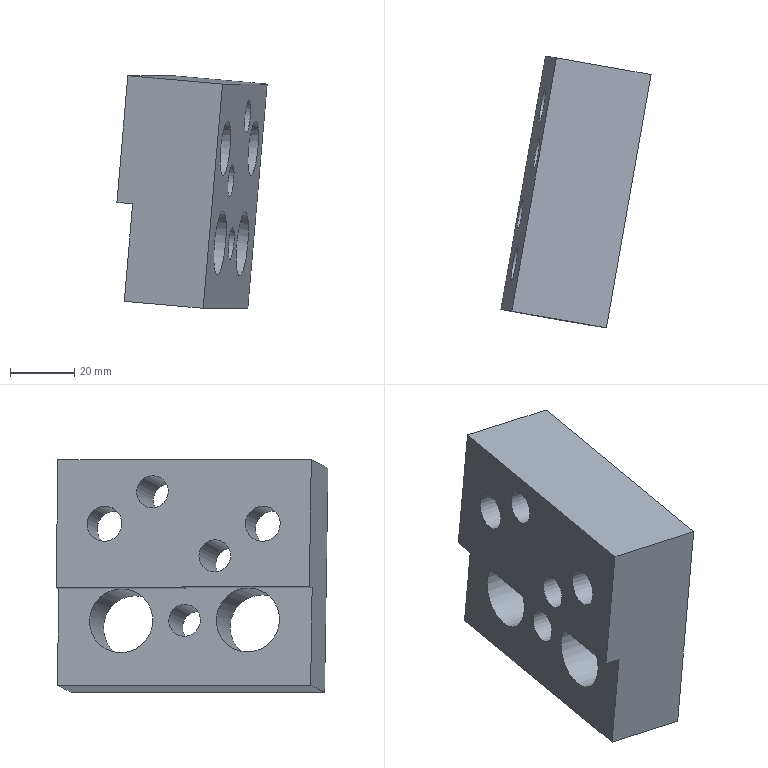Part | NX | features solid 2 | 1 solid | 21 faces | box 46.72 x 84.577 x 72.348 mm | volume 124632 mm3 | plane 11 | cylinder 10 | commonest cylinder face diameters 10 x3 11 x2 17 x2 20 x2 0.557 x1
STEP:
#1=CARTESIAN_POINT('',(413.654,2.711,48.436));
#2=VERTEX_POINT('',#1);
#3=CARTESIAN_POINT('',(412.178,-5.66,48.436));
#4=DIRECTION('',(0.9811,-0.173,-0.08716));
#5=DIRECTION('',(0.1736,0.9848,0.));
#6=AXIS2_PLACEMENT_3D('',#3,#4,#5);
#7=CIRCLE('',#6,8.5);
#8=EDGE_CURVE('',#2,#2,#7,.F.);
#9=ORIENTED_EDGE('',*,*,#8,.T.);
#10=EDGE_LOOP('',(#9));
#11=FACE_BOUND('',#10,.T.);
#12=CARTESIAN_POINT('',(422.336,51.951,48.436));
#13=VERTEX_POINT('',#12);
#14=CARTESIAN_POINT('',(420.86,43.58,48.436));
#15=DIRECTION('',(0.9811,-0.173,-0.08716));
#16=DIRECTION('',(0.1736,0.9848,0.));
#17=AXIS2_PLACEMENT_3D('',#14,#15,#16);
#18=CIRCLE('',#17,8.5);
#19=EDGE_CURVE('',#13,#13,#18,.F.);
#20=ORIENTED_EDGE('',*,*,#19,.T.);
#21=EDGE_LOOP('',(#20));
#22=FACE_BOUND('',#21,.T.);
#23=CARTESIAN_POINT('',(414.863,24.481,18.839));
#24=VERTEX_POINT('',#23);
#25=CARTESIAN_POINT('',(413.995,19.557,18.839));
#26=DIRECTION('',(0.9811,-0.173,-0.08716));
#27=DIRECTION('',(0.1736,0.9848,0.));
#28=AXIS2_PLACEMENT_3D('',#25,#26,#27);
#29=CIRCLE('',#28,5.);
#30=EDGE_CURVE('',#24,#24,#29,.T.);
#31=ORIENTED_EDGE('',*,*,#30,.F.);
#32=EDGE_LOOP('',(#31));
#33=FACE_BOUND('',#32,.T.);
#34=CARTESIAN_POINT('',(425.182,58.05,68.36));
#35=VERTEX_POINT('',#34);
#36=CARTESIAN_POINT('',(411.29,-20.735,68.36));
#37=VERTEX_POINT('',#36);
#38=CARTESIAN_POINT('',(425.182,58.05,68.36));
#39=DIRECTION('',(0.1736,0.9848,0.));
#40=VECTOR('',#39,1000.);
#41=LINE('',#38,#40);
#42=EDGE_CURVE('',#35,#37,#41,.F.);
#43=ORIENTED_EDGE('',*,*,#42,.T.);
#44=CARTESIAN_POINT('',(405.282,-19.675,-1.373));
#45=VERTEX_POINT('',#44);
#46=CARTESIAN_POINT('',(412.427,-20.935,81.56));
#47=DIRECTION('',(-0.08583,0.01513,-0.9962));
#48=VECTOR('',#47,1000.);
#49=LINE('',#46,#48);
#50=EDGE_CURVE('',#45,#37,#49,.F.);
#51=ORIENTED_EDGE('',*,*,#50,.F.);
#52=CARTESIAN_POINT('',(419.174,59.109,-1.373));
#53=VERTEX_POINT('',#52);
#54=CARTESIAN_POINT('',(419.174,59.109,-1.373));
#55=DIRECTION('',(0.1736,0.9848,0.));
#56=VECTOR('',#55,1000.);
#57=LINE('',#54,#56);
#58=EDGE_CURVE('',#45,#53,#57,.T.);
#59=ORIENTED_EDGE('',*,*,#58,.T.);
#60=CARTESIAN_POINT('',(421.813,58.644,29.261));
#61=DIRECTION('',(-0.08583,0.01513,-0.9962));
#62=VECTOR('',#61,1000.);
#63=LINE('',#60,#62);
#64=EDGE_CURVE('',#35,#53,#63,.T.);
#65=ORIENTED_EDGE('',*,*,#64,.F.);
#66=EDGE_LOOP('',(#43,#51,#59,#65));
#67=FACE_BOUND('',#66,.T.);
#68=CARTESIAN_POINT('',(419.192,49.1,18.7));
#69=VERTEX_POINT('',#68);
#70=CARTESIAN_POINT('',(417.455,39.252,18.7));
#71=DIRECTION('',(0.9811,-0.173,-0.08716));
#72=DIRECTION('',(0.1736,0.9848,0.));
#73=AXIS2_PLACEMENT_3D('',#70,#71,#72);
#74=CIRCLE('',#73,10.);
#75=EDGE_CURVE('',#69,#69,#74,.T.);
#76=ORIENTED_EDGE('',*,*,#75,.F.);
#77=EDGE_LOOP('',(#76));
#78=FACE_BOUND('',#77,.T.);
#79=CARTESIAN_POINT('',(412.271,9.711,18.977));
#80=VERTEX_POINT('',#79);
#81=CARTESIAN_POINT('',(410.535,-0.137,18.977));
#82=DIRECTION('',(0.9811,-0.173,-0.08716));
#83=DIRECTION('',(0.1736,0.9848,0.));
#84=AXIS2_PLACEMENT_3D('',#81,#82,#83);
#85=CIRCLE('',#84,10.);
#86=EDGE_CURVE('',#80,#80,#85,.T.);
#87=ORIENTED_EDGE('',*,*,#86,.F.);
#88=EDGE_LOOP('',(#87));
#89=FACE_BOUND('',#88,.T.);
#90=CARTESIAN_POINT('',(419.982,33.581,58.398));
#91=VERTEX_POINT('',#90);
#92=CARTESIAN_POINT('',(419.114,28.657,58.398));
#93=DIRECTION('',(0.9811,-0.173,-0.08716));
#94=DIRECTION('',(0.1736,0.9848,0.));
#95=AXIS2_PLACEMENT_3D('',#92,#93,#94);
#96=CIRCLE('',#95,5.);
#97=EDGE_CURVE('',#91,#91,#96,.T.);
#98=ORIENTED_EDGE('',*,*,#97,.F.);
#99=EDGE_LOOP('',(#98));
#100=FACE_BOUND('',#99,.T.);
#101=CARTESIAN_POINT('',(414.793,14.188,38.474));
#102=VERTEX_POINT('',#101);
#103=CARTESIAN_POINT('',(413.924,9.264,38.474));
#104=DIRECTION('',(0.9811,-0.173,-0.08716));
#105=DIRECTION('',(0.1736,0.9848,0.));
#106=AXIS2_PLACEMENT_3D('',#103,#104,#105);
#107=CIRCLE('',#106,5.);
#108=EDGE_CURVE('',#102,#102,#107,.T.);
#109=ORIENTED_EDGE('',*,*,#108,.F.);
#110=EDGE_LOOP('',(#109));
#111=FACE_BOUND('',#110,.T.);
#112=CARTESIAN_POINT('',(426.319,57.849,81.56));
#113=DIRECTION('',(-0.9811,0.173,0.08716));
#114=DIRECTION('',(-0.1736,-0.9848,0.));
#115=AXIS2_PLACEMENT_3D('',#112,#113,#114);
#116=PLANE('',#115);
#117=ADVANCED_FACE('',(#11,#22,#33,#67,#78,#89,#100,#111),#116,.F.);
#118=CARTESIAN_POINT('',(385.361,19.377,41.089));
#119=VERTEX_POINT('',#118);
#120=CARTESIAN_POINT('',(384.493,14.453,41.089));
#121=DIRECTION('',(0.9811,-0.173,-0.08716));
#122=DIRECTION('',(0.1736,0.9848,0.));
#123=AXIS2_PLACEMENT_3D('',#120,#121,#122);
#124=CIRCLE('',#123,5.);
#125=EDGE_CURVE('',#119,#119,#124,.F.);
#126=ORIENTED_EDGE('',*,*,#125,.T.);
#127=EDGE_LOOP('',(#126));
#128=FACE_BOUND('',#127,.T.);
#129=ORIENTED_EDGE('',*,*,#108,.T.);
#130=EDGE_LOOP('',(#129));
#131=FACE_BOUND('',#130,.T.);
#132=CARTESIAN_POINT('',(315.818,26.562,47.19));
#133=DIRECTION('',(0.9811,-0.173,-0.08716));
#134=DIRECTION('',(-0.1736,-0.9848,0.));
#135=AXIS2_PLACEMENT_3D('',#132,#133,#134);
#136=CYLINDRICAL_SURFACE('',#135,5.);
#137=ADVANCED_FACE('',(#128,#131),#136,.F.);
#138=CARTESIAN_POINT('',(390.55,38.771,61.013));
#139=VERTEX_POINT('',#138);
#140=CARTESIAN_POINT('',(389.682,33.847,61.013));
#141=DIRECTION('',(0.9811,-0.173,-0.08716));
#142=DIRECTION('',(0.1736,0.9848,0.));
#143=AXIS2_PLACEMENT_3D('',#140,#141,#142);
#144=CIRCLE('',#143,5.);
#145=EDGE_CURVE('',#139,#139,#144,.F.);
#146=ORIENTED_EDGE('',*,*,#145,.T.);
#147=EDGE_LOOP('',(#146));
#148=FACE_BOUND('',#147,.T.);
#149=ORIENTED_EDGE('',*,*,#97,.T.);
#150=EDGE_LOOP('',(#149));
#151=FACE_BOUND('',#150,.T.);
#152=CARTESIAN_POINT('',(321.008,45.956,67.114));
#153=DIRECTION('',(0.9811,-0.173,-0.08716));
#154=DIRECTION('',(-0.1736,-0.9848,0.));
#155=AXIS2_PLACEMENT_3D('',#152,#153,#154);
#156=CYLINDRICAL_SURFACE('',#155,5.);
#157=ADVANCED_FACE('',(#148,#151),#156,.F.);
#158=CARTESIAN_POINT('',(394.647,63.434,0.8055));
#159=VERTEX_POINT('',#158);
#160=CARTESIAN_POINT('',(380.755,-15.351,0.8055));
#161=VERTEX_POINT('',#160);
#162=CARTESIAN_POINT('',(394.647,63.434,0.8055));
#163=DIRECTION('',(-0.1736,-0.9848,0.));
#164=VECTOR('',#163,1000.);
#165=LINE('',#162,#164);
#166=EDGE_CURVE('',#159,#161,#165,.T.);
#167=ORIENTED_EDGE('',*,*,#166,.F.);
#168=CARTESIAN_POINT('',(419.174,59.109,-1.373));
#169=DIRECTION('',(-0.9811,0.173,0.08716));
#170=VECTOR('',#169,1000.);
#171=LINE('',#168,#170);
#172=EDGE_CURVE('',#53,#159,#171,.T.);
#173=ORIENTED_EDGE('',*,*,#172,.F.);
#174=ORIENTED_EDGE('',*,*,#58,.F.);
#175=CARTESIAN_POINT('',(405.282,-19.675,-1.373));
#176=DIRECTION('',(-0.9811,0.173,0.08716));
#177=VECTOR('',#176,1000.);
#178=LINE('',#175,#177);
#179=EDGE_CURVE('',#45,#161,#178,.T.);
#180=ORIENTED_EDGE('',*,*,#179,.T.);
#181=EDGE_LOOP('',(#167,#173,#174,#180));
#182=FACE_BOUND('',#181,.T.);
#183=CARTESIAN_POINT('',(419.174,59.109,-1.373));
#184=DIRECTION('',(-0.08583,0.01513,-0.9962));
#185=DIRECTION('',(0.9963,0.,-0.08584));
#186=AXIS2_PLACEMENT_3D('',#183,#184,#185);
#187=PLANE('',#186);
#188=ADVANCED_FACE('',(#182),#187,.T.);
#189=CARTESIAN_POINT('',(383.367,-15.811,31.118));
#190=VERTEX_POINT('',#189);
#191=CARTESIAN_POINT('',(366.201,-12.784,-168.121));
#192=DIRECTION('',(0.08583,-0.01513,0.9962));
#193=VECTOR('',#192,1000.);
#194=LINE('',#191,#193);
#195=EDGE_CURVE('',#161,#190,#194,.T.);
#196=ORIENTED_EDGE('',*,*,#195,.F.);
#197=ORIENTED_EDGE('',*,*,#179,.F.);
#198=ORIENTED_EDGE('',*,*,#50,.T.);
#199=CARTESIAN_POINT('',(381.858,-15.545,70.975));
#200=VERTEX_POINT('',#199);
#201=CARTESIAN_POINT('',(411.29,-20.735,68.36));
#202=DIRECTION('',(-0.9811,0.173,0.08716));
#203=VECTOR('',#202,1000.);
#204=LINE('',#201,#203);
#205=EDGE_CURVE('',#37,#200,#204,.T.);
#206=ORIENTED_EDGE('',*,*,#205,.T.);
#207=CARTESIAN_POINT('',(378.462,-14.946,31.554));
#208=VERTEX_POINT('',#207);
#209=CARTESIAN_POINT('',(382.995,-15.746,84.174));
#210=DIRECTION('',(-0.08583,0.01513,-0.9962));
#211=VECTOR('',#210,1000.);
#212=LINE('',#209,#211);
#213=EDGE_CURVE('',#208,#200,#212,.F.);
#214=ORIENTED_EDGE('',*,*,#213,.F.);
#215=CARTESIAN_POINT('',(407.893,-20.136,28.939));
#216=DIRECTION('',(0.9811,-0.173,-0.08716));
#217=VECTOR('',#216,1000.);
#218=LINE('',#215,#217);
#219=EDGE_CURVE('',#208,#190,#218,.T.);
#220=ORIENTED_EDGE('',*,*,#219,.T.);
#221=EDGE_LOOP('',(#196,#197,#198,#206,#214,#220));
#222=FACE_BOUND('',#221,.T.);
#223=CARTESIAN_POINT('',(412.427,-20.935,81.56));
#224=DIRECTION('',(0.1736,0.9848,0.));
#225=DIRECTION('',(0.9848,-0.1736,0.));
#226=AXIS2_PLACEMENT_3D('',#223,#224,#225);
#227=PLANE('',#226);
#228=ADVANCED_FACE('',(#222),#227,.F.);
#229=CARTESIAN_POINT('',(397.235,62.978,30.841));
#230=VERTEX_POINT('',#229);
#231=CARTESIAN_POINT('',(380.068,66.005,-168.398));
#232=DIRECTION('',(-0.08583,0.01513,-0.9962));
#233=VECTOR('',#232,1000.);
#234=LINE('',#231,#233);
#235=EDGE_CURVE('',#159,#230,#234,.F.);
#236=ORIENTED_EDGE('',*,*,#235,.T.);
#237=CARTESIAN_POINT('',(392.33,63.843,31.276));
#238=VERTEX_POINT('',#237);
#239=CARTESIAN_POINT('',(421.761,58.653,28.662));
#240=DIRECTION('',(-0.9811,0.173,0.08716));
#241=VECTOR('',#240,1000.);
#242=LINE('',#239,#241);
#243=EDGE_CURVE('',#238,#230,#242,.F.);
#244=ORIENTED_EDGE('',*,*,#243,.F.);
#245=CARTESIAN_POINT('',(395.75,63.239,70.975));
#246=VERTEX_POINT('',#245);
#247=CARTESIAN_POINT('',(392.381,63.833,31.876));
#248=DIRECTION('',(-0.08583,0.01513,-0.9962));
#249=VECTOR('',#248,1000.);
#250=LINE('',#247,#249);
#251=EDGE_CURVE('',#246,#238,#250,.T.);
#252=ORIENTED_EDGE('',*,*,#251,.F.);
#253=CARTESIAN_POINT('',(425.182,58.05,68.36));
#254=DIRECTION('',(-0.9811,0.173,0.08716));
#255=VECTOR('',#254,1000.);
#256=LINE('',#253,#255);
#257=EDGE_CURVE('',#35,#246,#256,.T.);
#258=ORIENTED_EDGE('',*,*,#257,.F.);
#259=ORIENTED_EDGE('',*,*,#64,.T.);
#260=ORIENTED_EDGE('',*,*,#172,.T.);
#261=EDGE_LOOP('',(#236,#244,#252,#258,#259,#260));
#262=FACE_BOUND('',#261,.T.);
#263=CARTESIAN_POINT('',(421.813,58.644,29.261));
#264=DIRECTION('',(-0.1736,-0.9848,0.));
#265=DIRECTION('',(-0.9848,0.1736,0.));
#266=AXIS2_PLACEMENT_3D('',#263,#264,#265);
#267=PLANE('',#266);
#268=ADVANCED_FACE('',(#262),#267,.F.);
#269=ORIENTED_EDGE('',*,*,#125,.F.);
#270=EDGE_LOOP('',(#269));
#271=FACE_BOUND('',#270,.T.);
#272=ORIENTED_EDGE('',*,*,#145,.F.);
#273=EDGE_LOOP('',(#272));
#274=FACE_BOUND('',#273,.T.);
#275=CARTESIAN_POINT('',(383.701,4.946,51.051));
#276=VERTEX_POINT('',#275);
#277=CARTESIAN_POINT('',(382.746,-0.4703,51.051));
#278=DIRECTION('',(0.9811,-0.173,-0.08716));
#279=DIRECTION('',(0.1736,0.9848,0.));
#280=AXIS2_PLACEMENT_3D('',#277,#278,#279);
#281=CIRCLE('',#280,5.5);
#282=EDGE_CURVE('',#276,#276,#281,.F.);
#283=ORIENTED_EDGE('',*,*,#282,.F.);
#284=EDGE_LOOP('',(#283));
#285=FACE_BOUND('',#284,.T.);
#286=CARTESIAN_POINT('',(392.384,54.187,51.051));
#287=VERTEX_POINT('',#286);
#288=CARTESIAN_POINT('',(391.429,48.77,51.051));
#289=DIRECTION('',(0.9811,-0.173,-0.08716));
#290=DIRECTION('',(0.1736,0.9848,0.));
#291=AXIS2_PLACEMENT_3D('',#288,#289,#290);
#292=CIRCLE('',#291,5.5);
#293=EDGE_CURVE('',#287,#287,#292,.F.);
#294=ORIENTED_EDGE('',*,*,#293,.F.);
#295=EDGE_LOOP('',(#294));
#296=FACE_BOUND('',#295,.T.);
#297=CARTESIAN_POINT('',(385.359,24.172,31.554));
#298=VERTEX_POINT('',#297);
#299=CARTESIAN_POINT('',(381.961,4.901,31.554));
#300=DIRECTION('',(0.1736,0.9848,0.));
#301=VECTOR('',#300,1000.);
#302=LINE('',#299,#301);
#303=EDGE_CURVE('',#208,#298,#302,.T.);
#304=ORIENTED_EDGE('',*,*,#303,.F.);
#305=ORIENTED_EDGE('',*,*,#213,.T.);
#306=CARTESIAN_POINT('',(395.75,63.239,70.975));
#307=DIRECTION('',(0.1736,0.9848,0.));
#308=VECTOR('',#307,1000.);
#309=LINE('',#306,#308);
#310=EDGE_CURVE('',#246,#200,#309,.F.);
#311=ORIENTED_EDGE('',*,*,#310,.F.);
#312=ORIENTED_EDGE('',*,*,#251,.T.);
#313=CARTESIAN_POINT('',(385.384,24.45,31.276));
#314=VERTEX_POINT('',#313);
#315=CARTESIAN_POINT('',(388.882,44.29,31.276));
#316=DIRECTION('',(0.1736,0.9848,0.000000001));
#317=VECTOR('',#316,1000.);
#318=LINE('',#315,#317);
#319=EDGE_CURVE('',#314,#238,#318,.T.);
#320=ORIENTED_EDGE('',*,*,#319,.F.);
#321=CARTESIAN_POINT('',(385.335,24.176,31.276));
#322=DIRECTION('',(0.9811,-0.173,-0.08716));
#323=DIRECTION('',(0.1736,0.9848,0.));
#324=AXIS2_PLACEMENT_3D('',#321,#322,#323);
#325=CIRCLE('',#324,0.2785);
#326=EDGE_CURVE('',#298,#314,#325,.F.);
#327=ORIENTED_EDGE('',*,*,#326,.F.);
#328=EDGE_LOOP('',(#304,#305,#311,#312,#320,#327));
#329=FACE_BOUND('',#328,.T.);
#330=CARTESIAN_POINT('',(396.887,63.039,84.174));
#331=DIRECTION('',(-0.9811,0.173,0.08716));
#332=DIRECTION('',(-0.1736,-0.9848,0.));
#333=AXIS2_PLACEMENT_3D('',#330,#331,#332);
#334=PLANE('',#333);
#335=ADVANCED_FACE('',(#271,#274,#285,#296,#329),#334,.T.);
#336=ORIENTED_EDGE('',*,*,#310,.T.);
#337=ORIENTED_EDGE('',*,*,#205,.F.);
#338=ORIENTED_EDGE('',*,*,#42,.F.);
#339=ORIENTED_EDGE('',*,*,#257,.T.);
#340=EDGE_LOOP('',(#336,#337,#338,#339));
#341=FACE_BOUND('',#340,.T.);
#342=CARTESIAN_POINT('',(425.182,58.05,68.36));
#343=DIRECTION('',(0.08583,-0.01513,0.9962));
#344=DIRECTION('',(-0.9963,0.,0.08584));
#345=AXIS2_PLACEMENT_3D('',#342,#343,#344);
#346=PLANE('',#345);
#347=ADVANCED_FACE('',(#341),#346,.T.);
#348=CARTESIAN_POINT('',(390.289,23.585,30.841));
#349=VERTEX_POINT('',#348);
#350=CARTESIAN_POINT('',(390.264,23.307,31.118));
#351=VERTEX_POINT('',#350);
#352=CARTESIAN_POINT('',(390.241,23.311,30.841));
#353=DIRECTION('',(0.9811,-0.173,-0.08716));
#354=DIRECTION('',(0.1736,0.9848,0.));
#355=AXIS2_PLACEMENT_3D('',#352,#353,#354);
#356=CIRCLE('',#355,0.2785);
#357=EDGE_CURVE('',#349,#351,#356,.T.);
#358=ORIENTED_EDGE('',*,*,#357,.F.);
#359=CARTESIAN_POINT('',(393.787,43.425,30.841));
#360=VERTEX_POINT('',#359);
#361=CARTESIAN_POINT('',(393.787,43.425,30.841));
#362=DIRECTION('',(0.1736,0.9848,0.000000001));
#363=VECTOR('',#362,1000.);
#364=LINE('',#361,#363);
#365=EDGE_CURVE('',#349,#360,#364,.T.);
#366=ORIENTED_EDGE('',*,*,#365,.T.);
#367=CARTESIAN_POINT('',(392.929,43.577,20.879));
#368=DIRECTION('',(0.9811,-0.173,-0.08716));
#369=DIRECTION('',(0.08583,-0.01513,0.9962));
#370=AXIS2_PLACEMENT_3D('',#367,#368,#369);
#371=CIRCLE('',#370,10.);
#372=EDGE_CURVE('',#360,#360,#371,.T.);
#373=ORIENTED_EDGE('',*,*,#372,.T.);
#374=CARTESIAN_POINT('',(393.787,43.425,30.841));
#375=DIRECTION('',(0.1736,0.9848,0.000000001));
#376=VECTOR('',#375,1000.);
#377=LINE('',#374,#376);
#378=EDGE_CURVE('',#360,#230,#377,.T.);
#379=ORIENTED_EDGE('',*,*,#378,.T.);
#380=ORIENTED_EDGE('',*,*,#235,.F.);
#381=ORIENTED_EDGE('',*,*,#166,.T.);
#382=ORIENTED_EDGE('',*,*,#195,.T.);
#383=CARTESIAN_POINT('',(386.867,4.036,31.118));
#384=VERTEX_POINT('',#383);
#385=CARTESIAN_POINT('',(386.867,4.036,31.118));
#386=DIRECTION('',(0.1736,0.9848,0.));
#387=VECTOR('',#386,1000.);
#388=LINE('',#385,#387);
#389=EDGE_CURVE('',#190,#384,#388,.T.);
#390=ORIENTED_EDGE('',*,*,#389,.T.);
#391=CARTESIAN_POINT('',(386.008,4.188,21.156));
#392=DIRECTION('',(0.9811,-0.173,-0.08716));
#393=DIRECTION('',(-0.08583,0.01513,-0.9962));
#394=AXIS2_PLACEMENT_3D('',#391,#392,#393);
#395=CIRCLE('',#394,10.);
#396=EDGE_CURVE('',#384,#384,#395,.T.);
#397=ORIENTED_EDGE('',*,*,#396,.T.);
#398=CARTESIAN_POINT('',(386.867,4.036,31.118));
#399=DIRECTION('',(0.1736,0.9848,0.));
#400=VECTOR('',#399,1000.);
#401=LINE('',#398,#400);
#402=EDGE_CURVE('',#384,#351,#401,.T.);
#403=ORIENTED_EDGE('',*,*,#402,.T.);
#404=EDGE_LOOP('',(#358,#366,#373,#379,#380,#381,#382,#390,#397,#403));
#405=FACE_BOUND('',#404,.T.);
#406=CARTESIAN_POINT('',(390.337,28.805,21.017));
#407=VERTEX_POINT('',#406);
#408=CARTESIAN_POINT('',(389.468,23.881,21.017));
#409=DIRECTION('',(0.9811,-0.173,-0.08716));
#410=DIRECTION('',(0.1736,0.9848,0.));
#411=AXIS2_PLACEMENT_3D('',#408,#409,#410);
#412=CIRCLE('',#411,5.);
#413=EDGE_CURVE('',#407,#407,#412,.T.);
#414=ORIENTED_EDGE('',*,*,#413,.T.);
#415=EDGE_LOOP('',(#414));
#416=FACE_BOUND('',#415,.T.);
#417=CARTESIAN_POINT('',(376.621,46.452,-168.398));
#418=DIRECTION('',(-0.9811,0.173,0.08716));
#419=DIRECTION('',(0.1736,0.9848,0.));
#420=AXIS2_PLACEMENT_3D('',#417,#418,#419);
#421=PLANE('',#420);
#422=ADVANCED_FACE('',(#405,#416),#421,.T.);
#423=ORIENTED_EDGE('',*,*,#365,.F.);
#424=CARTESIAN_POINT('',(414.815,19.261,28.662));
#425=DIRECTION('',(-0.9811,0.173,0.08716));
#426=VECTOR('',#425,1000.);
#427=LINE('',#424,#426);
#428=EDGE_CURVE('',#314,#349,#427,.F.);
#429=ORIENTED_EDGE('',*,*,#428,.F.);
#430=ORIENTED_EDGE('',*,*,#319,.T.);
#431=ORIENTED_EDGE('',*,*,#243,.T.);
#432=ORIENTED_EDGE('',*,*,#378,.F.);
#433=EDGE_LOOP('',(#423,#429,#430,#431,#432));
#434=FACE_BOUND('',#433,.T.);
#435=CARTESIAN_POINT('',(376.133,52.305,32.497));
#436=DIRECTION('',(-0.08583,0.01513,-0.9962));
#437=DIRECTION('',(0.9811,-0.173,-0.08716));
#438=AXIS2_PLACEMENT_3D('',#435,#436,#437);
#439=PLANE('',#438);
#440=ADVANCED_FACE('',(#434),#439,.T.);
#441=ORIENTED_EDGE('',*,*,#389,.F.);
#442=ORIENTED_EDGE('',*,*,#219,.F.);
#443=ORIENTED_EDGE('',*,*,#303,.T.);
#444=CARTESIAN_POINT('',(371.624,26.594,32.774));
#445=DIRECTION('',(-0.9811,0.173,0.08716));
#446=VECTOR('',#445,1000.);
#447=LINE('',#444,#446);
#448=EDGE_CURVE('',#351,#298,#447,.T.);
#449=ORIENTED_EDGE('',*,*,#448,.F.);
#450=ORIENTED_EDGE('',*,*,#402,.F.);
#451=EDGE_LOOP('',(#441,#442,#443,#449,#450));
#452=FACE_BOUND('',#451,.T.);
#453=CARTESIAN_POINT('',(369.213,12.916,32.774));
#454=DIRECTION('',(-0.08583,0.01513,-0.9962));
#455=DIRECTION('',(0.9811,-0.173,-0.08716));
#456=AXIS2_PLACEMENT_3D('',#453,#454,#455);
#457=PLANE('',#456);
#458=ADVANCED_FACE('',(#452),#457,.T.);
#459=ORIENTED_EDGE('',*,*,#326,.T.);
#460=ORIENTED_EDGE('',*,*,#428,.T.);
#461=ORIENTED_EDGE('',*,*,#357,.T.);
#462=ORIENTED_EDGE('',*,*,#448,.T.);
#463=EDGE_LOOP('',(#459,#460,#461,#462));
#464=FACE_BOUND('',#463,.T.);
#465=CARTESIAN_POINT('',(414.767,18.986,28.662));
#466=DIRECTION('',(-0.9811,0.173,0.08716));
#467=DIRECTION('',(0.1736,0.9848,0.));
#468=AXIS2_PLACEMENT_3D('',#465,#466,#467);
#469=CYLINDRICAL_SURFACE('',#468,0.2785);
#470=ADVANCED_FACE('',(#464),#469,.F.);
#471=ORIENTED_EDGE('',*,*,#75,.T.);
#472=EDGE_LOOP('',(#471));
#473=FACE_BOUND('',#472,.T.);
#474=ORIENTED_EDGE('',*,*,#372,.F.);
#475=EDGE_LOOP('',(#474));
#476=FACE_BOUND('',#475,.T.);
#477=CARTESIAN_POINT('',(378.213,46.172,22.186));
#478=DIRECTION('',(0.9811,-0.173,-0.08716));
#479=DIRECTION('',(0.08583,-0.01513,0.9962));
#480=AXIS2_PLACEMENT_3D('',#477,#478,#479);
#481=CYLINDRICAL_SURFACE('',#480,10.);
#482=ADVANCED_FACE('',(#473,#476),#481,.F.);
#483=ORIENTED_EDGE('',*,*,#30,.T.);
#484=EDGE_LOOP('',(#483));
#485=FACE_BOUND('',#484,.T.);
#486=ORIENTED_EDGE('',*,*,#413,.F.);
#487=EDGE_LOOP('',(#486));
#488=FACE_BOUND('',#487,.T.);
#489=CARTESIAN_POINT('',(374.753,26.476,22.325));
#490=DIRECTION('',(0.9811,-0.173,-0.08716));
#491=DIRECTION('',(-0.08583,0.01513,-0.9962));
#492=AXIS2_PLACEMENT_3D('',#489,#490,#491);
#493=CYLINDRICAL_SURFACE('',#492,5.);
#494=ADVANCED_FACE('',(#485,#488),#493,.F.);
#495=ORIENTED_EDGE('',*,*,#86,.T.);
#496=EDGE_LOOP('',(#495));
#497=FACE_BOUND('',#496,.T.);
#498=ORIENTED_EDGE('',*,*,#396,.F.);
#499=EDGE_LOOP('',(#498));
#500=FACE_BOUND('',#499,.T.);
#501=CARTESIAN_POINT('',(371.292,6.783,22.463));
#502=DIRECTION('',(0.9811,-0.173,-0.08716));
#503=DIRECTION('',(0.08583,-0.01513,0.9962));
#504=AXIS2_PLACEMENT_3D('',#501,#502,#503);
#505=CYLINDRICAL_SURFACE('',#504,10.);
#506=ADVANCED_FACE('',(#497,#500),#505,.F.);
#507=CARTESIAN_POINT('',(410.043,51.073,49.482));
#508=VERTEX_POINT('',#507);
#509=CARTESIAN_POINT('',(409.088,45.656,49.482));
#510=DIRECTION('',(0.9811,-0.173,-0.08716));
#511=DIRECTION('',(0.1736,0.9848,0.));
#512=AXIS2_PLACEMENT_3D('',#509,#510,#511);
#513=CIRCLE('',#512,5.5);
#514=EDGE_CURVE('',#508,#508,#513,.F.);
#515=ORIENTED_EDGE('',*,*,#514,.F.);
#516=EDGE_LOOP('',(#515));
#517=FACE_BOUND('',#516,.T.);
#518=ORIENTED_EDGE('',*,*,#293,.T.);
#519=EDGE_LOOP('',(#518));
#520=FACE_BOUND('',#519,.T.);
#521=CARTESIAN_POINT('',(373.769,51.884,52.62));
#522=DIRECTION('',(0.9811,-0.173,-0.08716));
#523=DIRECTION('',(-0.1736,-0.9848,0.));
#524=AXIS2_PLACEMENT_3D('',#521,#522,#523);
#525=CYLINDRICAL_SURFACE('',#524,5.5);
#526=ADVANCED_FACE('',(#517,#520),#525,.F.);
#527=ORIENTED_EDGE('',*,*,#514,.T.);
#528=EDGE_LOOP('',(#527));
#529=FACE_BOUND('',#528,.T.);
#530=CARTESIAN_POINT('',(407.612,37.285,49.482));
#531=VERTEX_POINT('',#530);
#532=CARTESIAN_POINT('',(409.088,45.656,49.482));
#533=DIRECTION('',(-0.9811,0.173,0.08716));
#534=DIRECTION('',(-0.1736,-0.9848,0.));
#535=AXIS2_PLACEMENT_3D('',#532,#533,#534);
#536=CIRCLE('',#535,8.5);
#537=EDGE_CURVE('',#531,#531,#536,.T.);
#538=ORIENTED_EDGE('',*,*,#537,.F.);
#539=EDGE_LOOP('',(#538));
#540=FACE_BOUND('',#539,.T.);
#541=CARTESIAN_POINT('',(409.088,45.656,49.482));
#542=DIRECTION('',(-0.9811,0.173,0.08716));
#543=DIRECTION('',(0.1736,0.9848,0.));
#544=AXIS2_PLACEMENT_3D('',#541,#542,#543);
#545=PLANE('',#544);
#546=ADVANCED_FACE('',(#529,#540),#545,.F.);
#547=ORIENTED_EDGE('',*,*,#19,.F.);
#548=EDGE_LOOP('',(#547));
#549=FACE_BOUND('',#548,.T.);
#550=ORIENTED_EDGE('',*,*,#537,.T.);
#551=EDGE_LOOP('',(#550));
#552=FACE_BOUND('',#551,.T.);
#553=CARTESIAN_POINT('',(409.088,45.656,49.482));
#554=DIRECTION('',(0.9811,-0.173,-0.08716));
#555=DIRECTION('',(-0.1736,-0.9848,0.));
#556=AXIS2_PLACEMENT_3D('',#553,#554,#555);
#557=CYLINDRICAL_SURFACE('',#556,8.5);
#558=ADVANCED_FACE('',(#549,#552),#557,.F.);
#559=CARTESIAN_POINT('',(401.36,1.832,49.482));
#560=VERTEX_POINT('',#559);
#561=CARTESIAN_POINT('',(400.405,-3.584,49.482));
#562=DIRECTION('',(0.9811,-0.173,-0.08716));
#563=DIRECTION('',(0.1736,0.9848,0.));
#564=AXIS2_PLACEMENT_3D('',#561,#562,#563);
#565=CIRCLE('',#564,5.5);
#566=EDGE_CURVE('',#560,#560,#565,.F.);
#567=ORIENTED_EDGE('',*,*,#566,.F.);
#568=EDGE_LOOP('',(#567));
#569=FACE_BOUND('',#568,.T.);
#570=ORIENTED_EDGE('',*,*,#282,.T.);
#571=EDGE_LOOP('',(#570));
#572=FACE_BOUND('',#571,.T.);
#573=CARTESIAN_POINT('',(365.087,2.643,52.62));
#574=DIRECTION('',(0.9811,-0.173,-0.08716));
#575=DIRECTION('',(-0.1736,-0.9848,0.));
#576=AXIS2_PLACEMENT_3D('',#573,#574,#575);
#577=CYLINDRICAL_SURFACE('',#576,5.5);
#578=ADVANCED_FACE('',(#569,#572),#577,.F.);
#579=ORIENTED_EDGE('',*,*,#566,.T.);
#580=EDGE_LOOP('',(#579));
#581=FACE_BOUND('',#580,.T.);
#582=CARTESIAN_POINT('',(398.929,-11.955,49.482));
#583=VERTEX_POINT('',#582);
#584=CARTESIAN_POINT('',(400.405,-3.584,49.482));
#585=DIRECTION('',(-0.9811,0.173,0.08716));
#586=DIRECTION('',(-0.1736,-0.9848,0.));
#587=AXIS2_PLACEMENT_3D('',#584,#585,#586);
#588=CIRCLE('',#587,8.5);
#589=EDGE_CURVE('',#583,#583,#588,.T.);
#590=ORIENTED_EDGE('',*,*,#589,.F.);
#591=EDGE_LOOP('',(#590));
#592=FACE_BOUND('',#591,.T.);
#593=CARTESIAN_POINT('',(400.405,-3.584,49.482));
#594=DIRECTION('',(-0.9811,0.173,0.08716));
#595=DIRECTION('',(0.1736,0.9848,0.));
#596=AXIS2_PLACEMENT_3D('',#593,#594,#595);
#597=PLANE('',#596);
#598=ADVANCED_FACE('',(#581,#592),#597,.F.);
#599=ORIENTED_EDGE('',*,*,#8,.F.);
#600=EDGE_LOOP('',(#599));
#601=FACE_BOUND('',#600,.T.);
#602=ORIENTED_EDGE('',*,*,#589,.T.);
#603=EDGE_LOOP('',(#602));
#604=FACE_BOUND('',#603,.T.);
#605=CARTESIAN_POINT('',(400.405,-3.584,49.482));
#606=DIRECTION('',(0.9811,-0.173,-0.08716));
#607=DIRECTION('',(-0.1736,-0.9848,0.));
#608=AXIS2_PLACEMENT_3D('',#605,#606,#607);
#609=CYLINDRICAL_SURFACE('',#608,8.5);
#610=ADVANCED_FACE('',(#601,#604),#609,.F.);
#611=CLOSED_SHELL('',(#117,#137,#157,#188,#228,#268,#335,#347,#422,#440,#458,#470,#482,#494,#506,#526,#546,#558,#578,#598,#610));
#612=MANIFOLD_SOLID_BREP('',#611);
#613=(LENGTH_UNIT()NAMED_UNIT(*)SI_UNIT(.MILLI.,.METRE.));
#614=UNCERTAINTY_MEASURE_WITH_UNIT(LENGTH_MEASURE(0.00001),#613,'','');
#615=(NAMED_UNIT(*)PLANE_ANGLE_UNIT()SI_UNIT($,.RADIAN.));
#616=(NAMED_UNIT(*)SI_UNIT($,.STERADIAN.)SOLID_ANGLE_UNIT());
#617=(GEOMETRIC_REPRESENTATION_CONTEXT(3)GLOBAL_UNCERTAINTY_ASSIGNED_CONTEXT((#614))GLOBAL_UNIT_ASSIGNED_CONTEXT((#613,#615,#616))REPRESENTATION_CONTEXT('',''));
#618=ADVANCED_BREP_SHAPE_REPRESENTATION('',(#612),#617);